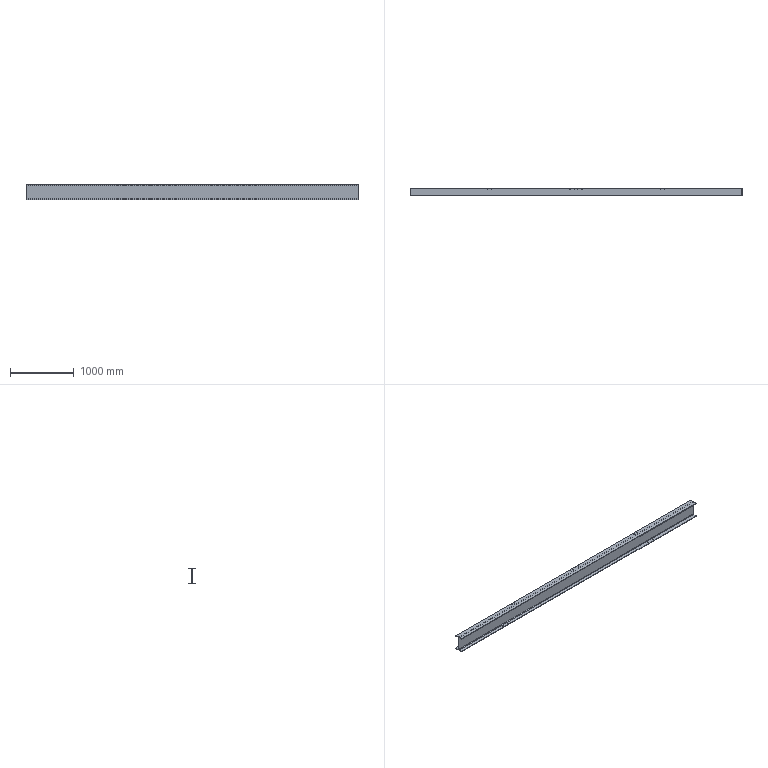Part | STEP file | PN_0031 main beam HN250X125=5225_Default<As Machined> | 1 solid | 36 faces | box 5225 x 125 x 250 mm | volume 19289440 mm3 | cylinder 20 | plane 16 | commonest cylinder face diameters 6.8 x8 18 x8 16 x4